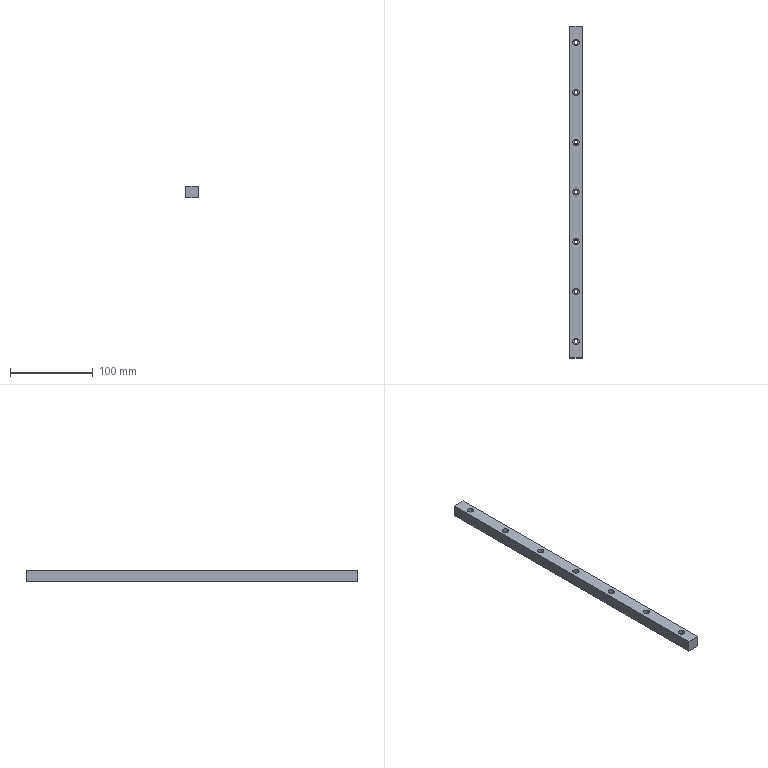Part | NX | 1 solid | 41 faces | box 15 x 400 x 14 mm | volume 81388 mm3 | cylinder 28 | plane 13 | commonest cylinder face diameters 4.5 x14 7.5 x12 8 x2
STEP:
#1=CARTESIAN_POINT('',(0.,-60.,0.));
#2=VERTEX_POINT('',#1);
#3=CARTESIAN_POINT('',(15.,-60.,0.));
#4=VERTEX_POINT('',#3);
#5=CARTESIAN_POINT('',(0.,-60.,0.));
#6=DIRECTION('',(1.,0.,0.));
#7=VECTOR('',#6,1000.);
#8=LINE('',#5,#7);
#9=EDGE_CURVE('',#2,#4,#8,.T.);
#10=ORIENTED_EDGE('',*,*,#9,.F.);
#11=CARTESIAN_POINT('',(0.,-60.,-14.));
#12=VERTEX_POINT('',#11);
#13=CARTESIAN_POINT('',(0.,-60.,0.));
#14=DIRECTION('',(0.,0.,1.));
#15=VECTOR('',#14,1000.);
#16=LINE('',#13,#15);
#17=EDGE_CURVE('',#12,#2,#16,.T.);
#18=ORIENTED_EDGE('',*,*,#17,.F.);
#19=CARTESIAN_POINT('',(15.,-60.,-14.));
#20=VERTEX_POINT('',#19);
#21=CARTESIAN_POINT('',(0.,-60.,-14.));
#22=DIRECTION('',(-1.,0.,0.));
#23=VECTOR('',#22,1000.);
#24=LINE('',#21,#23);
#25=EDGE_CURVE('',#20,#12,#24,.T.);
#26=ORIENTED_EDGE('',*,*,#25,.F.);
#27=CARTESIAN_POINT('',(15.,-60.,0.));
#28=DIRECTION('',(0.,0.,1.));
#29=VECTOR('',#28,1000.);
#30=LINE('',#27,#29);
#31=EDGE_CURVE('',#20,#4,#30,.T.);
#32=ORIENTED_EDGE('',*,*,#31,.T.);
#33=EDGE_LOOP('',(#10,#18,#26,#32));
#34=FACE_BOUND('',#33,.T.);
#35=CARTESIAN_POINT('',(76.5,-60.,-29.));
#36=DIRECTION('',(0.,-1.,0.));
#37=DIRECTION('',(0.,0.,-1.));
#38=AXIS2_PLACEMENT_3D('',#35,#36,#37);
#39=PLANE('',#38);
#40=ADVANCED_FACE('',(#34),#39,.T.);
#41=ORIENTED_EDGE('',*,*,#25,.T.);
#42=CARTESIAN_POINT('',(0.,340.,-14.));
#43=VERTEX_POINT('',#42);
#44=CARTESIAN_POINT('',(0.,0.,-14.));
#45=DIRECTION('',(0.,1.,0.));
#46=VECTOR('',#45,1000.);
#47=LINE('',#44,#46);
#48=EDGE_CURVE('',#12,#43,#47,.T.);
#49=ORIENTED_EDGE('',*,*,#48,.T.);
#50=CARTESIAN_POINT('',(15.,340.,-14.));
#51=VERTEX_POINT('',#50);
#52=CARTESIAN_POINT('',(0.,340.,-14.));
#53=DIRECTION('',(-1.,0.,0.));
#54=VECTOR('',#53,1000.);
#55=LINE('',#52,#54);
#56=EDGE_CURVE('',#51,#43,#55,.T.);
#57=ORIENTED_EDGE('',*,*,#56,.F.);
#58=CARTESIAN_POINT('',(15.,0.,-14.));
#59=DIRECTION('',(0.,-1.,0.));
#60=VECTOR('',#59,1000.);
#61=LINE('',#58,#60);
#62=EDGE_CURVE('',#51,#20,#61,.T.);
#63=ORIENTED_EDGE('',*,*,#62,.T.);
#64=EDGE_LOOP('',(#41,#49,#57,#63));
#65=FACE_BOUND('',#64,.T.);
#66=CARTESIAN_POINT('',(5.25,20.,-14.));
#67=VERTEX_POINT('',#66);
#68=CARTESIAN_POINT('',(9.75,20.,-14.));
#69=VERTEX_POINT('',#68);
#70=CARTESIAN_POINT('',(7.5,20.,-14.));
#71=DIRECTION('',(0.,0.,1.));
#72=DIRECTION('',(-1.,0.,0.));
#73=AXIS2_PLACEMENT_3D('',#70,#71,#72);
#74=CIRCLE('',#73,2.25);
#75=EDGE_CURVE('',#67,#69,#74,.T.);
#76=ORIENTED_EDGE('',*,*,#75,.T.);
#77=CARTESIAN_POINT('',(7.5,20.,-14.));
#78=DIRECTION('',(0.,0.,1.));
#79=DIRECTION('',(-1.,0.,0.));
#80=AXIS2_PLACEMENT_3D('',#77,#78,#79);
#81=CIRCLE('',#80,2.25);
#82=EDGE_CURVE('',#69,#67,#81,.T.);
#83=ORIENTED_EDGE('',*,*,#82,.T.);
#84=EDGE_LOOP('',(#76,#83));
#85=FACE_BOUND('',#84,.T.);
#86=CARTESIAN_POINT('',(5.25,320.,-14.));
#87=VERTEX_POINT('',#86);
#88=CARTESIAN_POINT('',(9.75,320.,-14.));
#89=VERTEX_POINT('',#88);
#90=CARTESIAN_POINT('',(7.5,320.,-14.));
#91=DIRECTION('',(0.,0.,1.));
#92=DIRECTION('',(-1.,0.,0.));
#93=AXIS2_PLACEMENT_3D('',#90,#91,#92);
#94=CIRCLE('',#93,2.25);
#95=EDGE_CURVE('',#87,#89,#94,.T.);
#96=ORIENTED_EDGE('',*,*,#95,.T.);
#97=CARTESIAN_POINT('',(7.5,320.,-14.));
#98=DIRECTION('',(0.,0.,1.));
#99=DIRECTION('',(-1.,0.,0.));
#100=AXIS2_PLACEMENT_3D('',#97,#98,#99);
#101=CIRCLE('',#100,2.25);
#102=EDGE_CURVE('',#89,#87,#101,.T.);
#103=ORIENTED_EDGE('',*,*,#102,.T.);
#104=EDGE_LOOP('',(#96,#103));
#105=FACE_BOUND('',#104,.T.);
#106=CARTESIAN_POINT('',(5.25,260.,-14.));
#107=VERTEX_POINT('',#106);
#108=CARTESIAN_POINT('',(9.75,260.,-14.));
#109=VERTEX_POINT('',#108);
#110=CARTESIAN_POINT('',(7.5,260.,-14.));
#111=DIRECTION('',(0.,0.,1.));
#112=DIRECTION('',(-1.,0.,0.));
#113=AXIS2_PLACEMENT_3D('',#110,#111,#112);
#114=CIRCLE('',#113,2.25);
#115=EDGE_CURVE('',#107,#109,#114,.T.);
#116=ORIENTED_EDGE('',*,*,#115,.T.);
#117=CARTESIAN_POINT('',(7.5,260.,-14.));
#118=DIRECTION('',(0.,0.,1.));
#119=DIRECTION('',(-1.,0.,0.));
#120=AXIS2_PLACEMENT_3D('',#117,#118,#119);
#121=CIRCLE('',#120,2.25);
#122=EDGE_CURVE('',#109,#107,#121,.T.);
#123=ORIENTED_EDGE('',*,*,#122,.T.);
#124=EDGE_LOOP('',(#116,#123));
#125=FACE_BOUND('',#124,.T.);
#126=CARTESIAN_POINT('',(9.75,200.,-14.));
#127=VERTEX_POINT('',#126);
#128=CARTESIAN_POINT('',(5.25,200.,-14.));
#129=VERTEX_POINT('',#128);
#130=CARTESIAN_POINT('',(7.5,200.,-14.));
#131=DIRECTION('',(0.,0.,1.));
#132=DIRECTION('',(-1.,0.,0.));
#133=AXIS2_PLACEMENT_3D('',#130,#131,#132);
#134=CIRCLE('',#133,2.25);
#135=EDGE_CURVE('',#127,#129,#134,.T.);
#136=ORIENTED_EDGE('',*,*,#135,.T.);
#137=CARTESIAN_POINT('',(7.5,200.,-14.));
#138=DIRECTION('',(0.,0.,1.));
#139=DIRECTION('',(-1.,0.,0.));
#140=AXIS2_PLACEMENT_3D('',#137,#138,#139);
#141=CIRCLE('',#140,2.25);
#142=EDGE_CURVE('',#129,#127,#141,.T.);
#143=ORIENTED_EDGE('',*,*,#142,.T.);
#144=EDGE_LOOP('',(#136,#143));
#145=FACE_BOUND('',#144,.T.);
#146=CARTESIAN_POINT('',(9.75,140.,-14.));
#147=VERTEX_POINT('',#146);
#148=CARTESIAN_POINT('',(5.25,140.,-14.));
#149=VERTEX_POINT('',#148);
#150=CARTESIAN_POINT('',(7.5,140.,-14.));
#151=DIRECTION('',(0.,0.,1.));
#152=DIRECTION('',(-1.,0.,0.));
#153=AXIS2_PLACEMENT_3D('',#150,#151,#152);
#154=CIRCLE('',#153,2.25);
#155=EDGE_CURVE('',#147,#149,#154,.T.);
#156=ORIENTED_EDGE('',*,*,#155,.T.);
#157=CARTESIAN_POINT('',(7.5,140.,-14.));
#158=DIRECTION('',(0.,0.,1.));
#159=DIRECTION('',(-1.,0.,0.));
#160=AXIS2_PLACEMENT_3D('',#157,#158,#159);
#161=CIRCLE('',#160,2.25);
#162=EDGE_CURVE('',#149,#147,#161,.T.);
#163=ORIENTED_EDGE('',*,*,#162,.T.);
#164=EDGE_LOOP('',(#156,#163));
#165=FACE_BOUND('',#164,.T.);
#166=CARTESIAN_POINT('',(9.75,80.,-14.));
#167=VERTEX_POINT('',#166);
#168=CARTESIAN_POINT('',(5.25,80.,-14.));
#169=VERTEX_POINT('',#168);
#170=CARTESIAN_POINT('',(7.5,80.,-14.));
#171=DIRECTION('',(0.,0.,1.));
#172=DIRECTION('',(-1.,0.,0.));
#173=AXIS2_PLACEMENT_3D('',#170,#171,#172);
#174=CIRCLE('',#173,2.25);
#175=EDGE_CURVE('',#167,#169,#174,.T.);
#176=ORIENTED_EDGE('',*,*,#175,.T.);
#177=CARTESIAN_POINT('',(7.5,80.,-14.));
#178=DIRECTION('',(0.,0.,1.));
#179=DIRECTION('',(-1.,0.,0.));
#180=AXIS2_PLACEMENT_3D('',#177,#178,#179);
#181=CIRCLE('',#180,2.25);
#182=EDGE_CURVE('',#169,#167,#181,.T.);
#183=ORIENTED_EDGE('',*,*,#182,.T.);
#184=EDGE_LOOP('',(#176,#183));
#185=FACE_BOUND('',#184,.T.);
#186=CARTESIAN_POINT('',(9.75,-40.,-14.));
#187=VERTEX_POINT('',#186);
#188=CARTESIAN_POINT('',(5.25,-40.,-14.));
#189=VERTEX_POINT('',#188);
#190=CARTESIAN_POINT('',(7.5,-40.,-14.));
#191=DIRECTION('',(0.,0.,1.));
#192=DIRECTION('',(1.,0.,0.));
#193=AXIS2_PLACEMENT_3D('',#190,#191,#192);
#194=CIRCLE('',#193,2.25);
#195=EDGE_CURVE('',#187,#189,#194,.T.);
#196=ORIENTED_EDGE('',*,*,#195,.T.);
#197=CARTESIAN_POINT('',(7.5,-40.,-14.));
#198=DIRECTION('',(0.,0.,1.));
#199=DIRECTION('',(1.,0.,0.));
#200=AXIS2_PLACEMENT_3D('',#197,#198,#199);
#201=CIRCLE('',#200,2.25);
#202=EDGE_CURVE('',#189,#187,#201,.T.);
#203=ORIENTED_EDGE('',*,*,#202,.T.);
#204=EDGE_LOOP('',(#196,#203));
#205=FACE_BOUND('',#204,.T.);
#206=CARTESIAN_POINT('',(15.,0.,-14.));
#207=DIRECTION('',(0.,0.,-1.));
#208=DIRECTION('',(0.,-1.,0.));
#209=AXIS2_PLACEMENT_3D('',#206,#207,#208);
#210=PLANE('',#209);
#211=ADVANCED_FACE('',(#65,#85,#105,#125,#145,#165,#185,#205),#210,.T.);
#212=ORIENTED_EDGE('',*,*,#17,.T.);
#213=CARTESIAN_POINT('',(0.,340.,0.));
#214=VERTEX_POINT('',#213);
#215=CARTESIAN_POINT('',(0.,0.,0.));
#216=DIRECTION('',(0.,1.,0.));
#217=VECTOR('',#216,1000.);
#218=LINE('',#215,#217);
#219=EDGE_CURVE('',#2,#214,#218,.T.);
#220=ORIENTED_EDGE('',*,*,#219,.T.);
#221=CARTESIAN_POINT('',(0.,340.,0.));
#222=DIRECTION('',(0.,0.,1.));
#223=VECTOR('',#222,1000.);
#224=LINE('',#221,#223);
#225=EDGE_CURVE('',#43,#214,#224,.T.);
#226=ORIENTED_EDGE('',*,*,#225,.F.);
#227=ORIENTED_EDGE('',*,*,#48,.F.);
#228=EDGE_LOOP('',(#212,#220,#226,#227));
#229=FACE_BOUND('',#228,.T.);
#230=CARTESIAN_POINT('',(0.,0.,-14.));
#231=DIRECTION('',(-1.,0.,0.));
#232=DIRECTION('',(0.,0.,1.));
#233=AXIS2_PLACEMENT_3D('',#230,#231,#232);
#234=PLANE('',#233);
#235=ADVANCED_FACE('',(#229),#234,.T.);
#236=ORIENTED_EDGE('',*,*,#9,.T.);
#237=CARTESIAN_POINT('',(15.,340.,0.));
#238=VERTEX_POINT('',#237);
#239=CARTESIAN_POINT('',(15.,0.,0.));
#240=DIRECTION('',(0.,1.,0.));
#241=VECTOR('',#240,1000.);
#242=LINE('',#239,#241);
#243=EDGE_CURVE('',#4,#238,#242,.T.);
#244=ORIENTED_EDGE('',*,*,#243,.T.);
#245=CARTESIAN_POINT('',(0.,340.,0.));
#246=DIRECTION('',(1.,0.,0.));
#247=VECTOR('',#246,1000.);
#248=LINE('',#245,#247);
#249=EDGE_CURVE('',#214,#238,#248,.T.);
#250=ORIENTED_EDGE('',*,*,#249,.F.);
#251=ORIENTED_EDGE('',*,*,#219,.F.);
#252=EDGE_LOOP('',(#236,#244,#250,#251));
#253=FACE_BOUND('',#252,.T.);
#254=CARTESIAN_POINT('',(11.25,20.,0.));
#255=VERTEX_POINT('',#254);
#256=CARTESIAN_POINT('',(3.75,20.,0.));
#257=VERTEX_POINT('',#256);
#258=CARTESIAN_POINT('',(7.5,20.,0.));
#259=DIRECTION('',(0.,0.,1.));
#260=DIRECTION('',(-1.,0.,0.));
#261=AXIS2_PLACEMENT_3D('',#258,#259,#260);
#262=CIRCLE('',#261,3.75);
#263=EDGE_CURVE('',#255,#257,#262,.T.);
#264=ORIENTED_EDGE('',*,*,#263,.F.);
#265=CARTESIAN_POINT('',(7.5,20.,0.));
#266=DIRECTION('',(0.,0.,1.));
#267=DIRECTION('',(-1.,0.,0.));
#268=AXIS2_PLACEMENT_3D('',#265,#266,#267);
#269=CIRCLE('',#268,3.75);
#270=EDGE_CURVE('',#257,#255,#269,.T.);
#271=ORIENTED_EDGE('',*,*,#270,.F.);
#272=EDGE_LOOP('',(#264,#271));
#273=FACE_BOUND('',#272,.T.);
#274=CARTESIAN_POINT('',(11.25,320.,0.));
#275=VERTEX_POINT('',#274);
#276=CARTESIAN_POINT('',(3.75,320.,0.));
#277=VERTEX_POINT('',#276);
#278=CARTESIAN_POINT('',(7.5,320.,0.));
#279=DIRECTION('',(0.,0.,1.));
#280=DIRECTION('',(-1.,0.,0.));
#281=AXIS2_PLACEMENT_3D('',#278,#279,#280);
#282=CIRCLE('',#281,3.75);
#283=EDGE_CURVE('',#275,#277,#282,.T.);
#284=ORIENTED_EDGE('',*,*,#283,.F.);
#285=CARTESIAN_POINT('',(7.5,320.,0.));
#286=DIRECTION('',(0.,0.,1.));
#287=DIRECTION('',(-1.,0.,0.));
#288=AXIS2_PLACEMENT_3D('',#285,#286,#287);
#289=CIRCLE('',#288,3.75);
#290=EDGE_CURVE('',#277,#275,#289,.T.);
#291=ORIENTED_EDGE('',*,*,#290,.F.);
#292=EDGE_LOOP('',(#284,#291));
#293=FACE_BOUND('',#292,.T.);
#294=CARTESIAN_POINT('',(11.25,260.,0.));
#295=VERTEX_POINT('',#294);
#296=CARTESIAN_POINT('',(3.75,260.,0.));
#297=VERTEX_POINT('',#296);
#298=CARTESIAN_POINT('',(7.5,260.,0.));
#299=DIRECTION('',(0.,0.,1.));
#300=DIRECTION('',(-1.,0.,0.));
#301=AXIS2_PLACEMENT_3D('',#298,#299,#300);
#302=CIRCLE('',#301,3.75);
#303=EDGE_CURVE('',#295,#297,#302,.T.);
#304=ORIENTED_EDGE('',*,*,#303,.F.);
#305=CARTESIAN_POINT('',(7.5,260.,0.));
#306=DIRECTION('',(0.,0.,1.));
#307=DIRECTION('',(-1.,0.,0.));
#308=AXIS2_PLACEMENT_3D('',#305,#306,#307);
#309=CIRCLE('',#308,3.75);
#310=EDGE_CURVE('',#297,#295,#309,.T.);
#311=ORIENTED_EDGE('',*,*,#310,.F.);
#312=EDGE_LOOP('',(#304,#311));
#313=FACE_BOUND('',#312,.T.);
#314=CARTESIAN_POINT('',(11.25,200.,0.));
#315=VERTEX_POINT('',#314);
#316=CARTESIAN_POINT('',(3.75,200.,0.));
#317=VERTEX_POINT('',#316);
#318=CARTESIAN_POINT('',(7.5,200.,0.));
#319=DIRECTION('',(0.,0.,1.));
#320=DIRECTION('',(-1.,0.,0.));
#321=AXIS2_PLACEMENT_3D('',#318,#319,#320);
#322=CIRCLE('',#321,3.75);
#323=EDGE_CURVE('',#315,#317,#322,.T.);
#324=ORIENTED_EDGE('',*,*,#323,.F.);
#325=CARTESIAN_POINT('',(7.5,200.,0.));
#326=DIRECTION('',(0.,0.,1.));
#327=DIRECTION('',(-1.,0.,0.));
#328=AXIS2_PLACEMENT_3D('',#325,#326,#327);
#329=CIRCLE('',#328,3.75);
#330=EDGE_CURVE('',#317,#315,#329,.T.);
#331=ORIENTED_EDGE('',*,*,#330,.F.);
#332=EDGE_LOOP('',(#324,#331));
#333=FACE_BOUND('',#332,.T.);
#334=CARTESIAN_POINT('',(11.25,140.,0.));
#335=VERTEX_POINT('',#334);
#336=CARTESIAN_POINT('',(3.75,140.,0.));
#337=VERTEX_POINT('',#336);
#338=CARTESIAN_POINT('',(7.5,140.,0.));
#339=DIRECTION('',(0.,0.,1.));
#340=DIRECTION('',(-1.,0.,0.));
#341=AXIS2_PLACEMENT_3D('',#338,#339,#340);
#342=CIRCLE('',#341,3.75);
#343=EDGE_CURVE('',#335,#337,#342,.T.);
#344=ORIENTED_EDGE('',*,*,#343,.F.);
#345=CARTESIAN_POINT('',(7.5,140.,0.));
#346=DIRECTION('',(0.,0.,1.));
#347=DIRECTION('',(-1.,0.,0.));
#348=AXIS2_PLACEMENT_3D('',#345,#346,#347);
#349=CIRCLE('',#348,3.75);
#350=EDGE_CURVE('',#337,#335,#349,.T.);
#351=ORIENTED_EDGE('',*,*,#350,.F.);
#352=EDGE_LOOP('',(#344,#351));
#353=FACE_BOUND('',#352,.T.);
#354=CARTESIAN_POINT('',(11.25,80.,0.));
#355=VERTEX_POINT('',#354);
#356=CARTESIAN_POINT('',(3.75,80.,0.));
#357=VERTEX_POINT('',#356);
#358=CARTESIAN_POINT('',(7.5,80.,0.));
#359=DIRECTION('',(0.,0.,1.));
#360=DIRECTION('',(-1.,0.,0.));
#361=AXIS2_PLACEMENT_3D('',#358,#359,#360);
#362=CIRCLE('',#361,3.75);
#363=EDGE_CURVE('',#355,#357,#362,.T.);
#364=ORIENTED_EDGE('',*,*,#363,.F.);
#365=CARTESIAN_POINT('',(7.5,80.,0.));
#366=DIRECTION('',(0.,0.,1.));
#367=DIRECTION('',(-1.,0.,0.));
#368=AXIS2_PLACEMENT_3D('',#365,#366,#367);
#369=CIRCLE('',#368,3.75);
#370=EDGE_CURVE('',#357,#355,#369,.T.);
#371=ORIENTED_EDGE('',*,*,#370,.F.);
#372=EDGE_LOOP('',(#364,#371));
#373=FACE_BOUND('',#372,.T.);
#374=CARTESIAN_POINT('',(3.5,-40.,0.));
#375=VERTEX_POINT('',#374);
#376=CARTESIAN_POINT('',(11.5,-40.,0.));
#377=VERTEX_POINT('',#376);
#378=CARTESIAN_POINT('',(7.5,-40.,0.));
#379=DIRECTION('',(0.,0.,1.));
#380=DIRECTION('',(1.,0.,0.));
#381=AXIS2_PLACEMENT_3D('',#378,#379,#380);
#382=CIRCLE('',#381,4.);
#383=EDGE_CURVE('',#375,#377,#382,.T.);
#384=ORIENTED_EDGE('',*,*,#383,.F.);
#385=CARTESIAN_POINT('',(7.5,-40.,0.));
#386=DIRECTION('',(0.,0.,1.));
#387=DIRECTION('',(1.,0.,0.));
#388=AXIS2_PLACEMENT_3D('',#385,#386,#387);
#389=CIRCLE('',#388,4.);
#390=EDGE_CURVE('',#377,#375,#389,.T.);
#391=ORIENTED_EDGE('',*,*,#390,.F.);
#392=EDGE_LOOP('',(#384,#391));
#393=FACE_BOUND('',#392,.T.);
#394=CARTESIAN_POINT('',(0.,0.,0.));
#395=DIRECTION('',(0.,0.,1.));
#396=DIRECTION('',(1.,0.,0.));
#397=AXIS2_PLACEMENT_3D('',#394,#395,#396);
#398=PLANE('',#397);
#399=ADVANCED_FACE('',(#253,#273,#293,#313,#333,#353,#373,#393),#398,.T.);
#400=ORIENTED_EDGE('',*,*,#31,.F.);
#401=ORIENTED_EDGE('',*,*,#62,.F.);
#402=CARTESIAN_POINT('',(15.,340.,0.));
#403=DIRECTION('',(0.,0.,-1.));
#404=VECTOR('',#403,1000.);
#405=LINE('',#402,#404);
#406=EDGE_CURVE('',#238,#51,#405,.T.);
#407=ORIENTED_EDGE('',*,*,#406,.F.);
#408=ORIENTED_EDGE('',*,*,#243,.F.);
#409=EDGE_LOOP('',(#400,#401,#407,#408));
#410=FACE_BOUND('',#409,.T.);
#411=CARTESIAN_POINT('',(15.,0.,0.));
#412=DIRECTION('',(1.,0.,0.));
#413=DIRECTION('',(0.,1.,0.));
#414=AXIS2_PLACEMENT_3D('',#411,#412,#413);
#415=PLANE('',#414);
#416=ADVANCED_FACE('',(#410),#415,.T.);
#417=ORIENTED_EDGE('',*,*,#249,.T.);
#418=ORIENTED_EDGE('',*,*,#406,.T.);
#419=ORIENTED_EDGE('',*,*,#56,.T.);
#420=ORIENTED_EDGE('',*,*,#225,.T.);
#421=EDGE_LOOP('',(#417,#418,#419,#420));
#422=FACE_BOUND('',#421,.T.);
#423=CARTESIAN_POINT('',(0.,340.,0.));
#424=DIRECTION('',(0.,1.,0.));
#425=DIRECTION('',(1.,0.,0.));
#426=AXIS2_PLACEMENT_3D('',#423,#424,#425);
#427=PLANE('',#426);
#428=ADVANCED_FACE('',(#422),#427,.T.);
#429=CARTESIAN_POINT('',(9.75,20.,-5.3));
#430=VERTEX_POINT('',#429);
#431=CARTESIAN_POINT('',(5.25,20.,-5.3));
#432=VERTEX_POINT('',#431);
#433=CARTESIAN_POINT('',(7.5,20.,-5.3));
#434=DIRECTION('',(0.,0.,1.));
#435=DIRECTION('',(1.,0.,0.));
#436=AXIS2_PLACEMENT_3D('',#433,#434,#435);
#437=CIRCLE('',#436,2.25);
#438=EDGE_CURVE('',#430,#432,#437,.T.);
#439=ORIENTED_EDGE('',*,*,#438,.T.);
#440=CARTESIAN_POINT('',(5.25,20.,-16.17));
#441=DIRECTION('',(0.,0.,1.));
#442=VECTOR('',#441,1000.);
#443=LINE('',#440,#442);
#444=EDGE_CURVE('',#432,#67,#443,.F.);
#445=ORIENTED_EDGE('',*,*,#444,.T.);
#446=ORIENTED_EDGE('',*,*,#82,.F.);
#447=CARTESIAN_POINT('',(9.75,20.,-16.17));
#448=DIRECTION('',(0.,0.,1.));
#449=VECTOR('',#448,1000.);
#450=LINE('',#447,#449);
#451=EDGE_CURVE('',#430,#69,#450,.F.);
#452=ORIENTED_EDGE('',*,*,#451,.F.);
#453=EDGE_LOOP('',(#439,#445,#446,#452));
#454=FACE_BOUND('',#453,.T.);
#455=CARTESIAN_POINT('',(7.5,20.,-16.17));
#456=DIRECTION('',(0.,0.,1.));
#457=DIRECTION('',(-1.,0.,0.));
#458=AXIS2_PLACEMENT_3D('',#455,#456,#457);
#459=CYLINDRICAL_SURFACE('',#458,2.25);
#460=ADVANCED_FACE('',(#454),#459,.F.);
#461=ORIENTED_EDGE('',*,*,#115,.F.);
#462=CARTESIAN_POINT('',(5.25,260.,-5.3));
#463=VERTEX_POINT('',#462);
#464=CARTESIAN_POINT('',(5.25,260.,-16.17));
#465=DIRECTION('',(0.,0.,1.));
#466=VECTOR('',#465,1000.);
#467=LINE('',#464,#466);
#468=EDGE_CURVE('',#463,#107,#467,.F.);
#469=ORIENTED_EDGE('',*,*,#468,.F.);
#470=CARTESIAN_POINT('',(9.75,260.,-5.3));
#471=VERTEX_POINT('',#470);
#472=CARTESIAN_POINT('',(7.5,260.,-5.3));
#473=DIRECTION('',(0.,0.,1.));
#474=DIRECTION('',(-1.,0.,0.));
#475=AXIS2_PLACEMENT_3D('',#472,#473,#474);
#476=CIRCLE('',#475,2.25);
#477=EDGE_CURVE('',#463,#471,#476,.T.);
#478=ORIENTED_EDGE('',*,*,#477,.T.);
#479=CARTESIAN_POINT('',(9.75,260.,-16.17));
#480=DIRECTION('',(0.,0.,1.));
#481=VECTOR('',#480,1000.);
#482=LINE('',#479,#481);
#483=EDGE_CURVE('',#471,#109,#482,.F.);
#484=ORIENTED_EDGE('',*,*,#483,.T.);
#485=EDGE_LOOP('',(#461,#469,#478,#484));
#486=FACE_BOUND('',#485,.T.);
#487=CARTESIAN_POINT('',(7.5,260.,-16.17));
#488=DIRECTION('',(0.,0.,1.));
#489=DIRECTION('',(-1.,0.,0.));
#490=AXIS2_PLACEMENT_3D('',#487,#488,#489);
#491=CYLINDRICAL_SURFACE('',#490,2.25);
#492=ADVANCED_FACE('',(#486),#491,.F.);
#493=CARTESIAN_POINT('',(11.25,20.,-5.3));
#494=VERTEX_POINT('',#493);
#495=CARTESIAN_POINT('',(3.75,20.,-5.3));
#496=VERTEX_POINT('',#495);
#497=CARTESIAN_POINT('',(7.5,20.,-5.3));
#498=DIRECTION('',(0.,0.,-1.));
#499=DIRECTION('',(-1.,0.,0.));
#500=AXIS2_PLACEMENT_3D('',#497,#498,#499);
#501=CIRCLE('',#500,3.75);
#502=EDGE_CURVE('',#494,#496,#501,.T.);
#503=ORIENTED_EDGE('',*,*,#502,.F.);
#504=CARTESIAN_POINT('',(7.5,20.,-5.3));
#505=DIRECTION('',(0.,0.,-1.));
#506=DIRECTION('',(-1.,0.,0.));
#507=AXIS2_PLACEMENT_3D('',#504,#505,#506);
#508=CIRCLE('',#507,3.75);
#509=EDGE_CURVE('',#496,#494,#508,.T.);
#510=ORIENTED_EDGE('',*,*,#509,.F.);
#511=EDGE_LOOP('',(#503,#510));
#512=FACE_BOUND('',#511,.T.);
#513=ORIENTED_EDGE('',*,*,#438,.F.);
#514=CARTESIAN_POINT('',(7.5,20.,-5.3));
#515=DIRECTION('',(0.,0.,1.));
#516=DIRECTION('',(1.,0.,0.));
#517=AXIS2_PLACEMENT_3D('',#514,#515,#516);
#518=CIRCLE('',#517,2.25);
#519=EDGE_CURVE('',#432,#430,#518,.T.);
#520=ORIENTED_EDGE('',*,*,#519,.F.);
#521=EDGE_LOOP('',(#513,#520));
#522=FACE_BOUND('',#521,.T.);
#523=CARTESIAN_POINT('',(7.5,20.,-5.3));
#524=DIRECTION('',(0.,0.,1.));
#525=DIRECTION('',(1.,0.,0.));
#526=AXIS2_PLACEMENT_3D('',#523,#524,#525);
#527=PLANE('',#526);
#528=ADVANCED_FACE('',(#512,#522),#527,.T.);
#529=ORIENTED_EDGE('',*,*,#502,.T.);
#530=CARTESIAN_POINT('',(3.75,20.,-16.17));
#531=DIRECTION('',(0.,0.,1.));
#532=VECTOR('',#531,1000.);
#533=LINE('',#530,#532);
#534=EDGE_CURVE('',#257,#496,#533,.F.);
#535=ORIENTED_EDGE('',*,*,#534,.F.);
#536=ORIENTED_EDGE('',*,*,#270,.T.);
#537=CARTESIAN_POINT('',(11.25,20.,-16.17));
#538=DIRECTION('',(0.,0.,1.));
#539=VECTOR('',#538,1000.);
#540=LINE('',#537,#539);
#541=EDGE_CURVE('',#255,#494,#540,.F.);
#542=ORIENTED_EDGE('',*,*,#541,.T.);
#543=EDGE_LOOP('',(#529,#535,#536,#542));
#544=FACE_BOUND('',#543,.T.);
#545=CARTESIAN_POINT('',(7.5,20.,-16.17));
#546=DIRECTION('',(0.,0.,1.));
#547=DIRECTION('',(-1.,0.,0.));
#548=AXIS2_PLACEMENT_3D('',#545,#546,#547);
#549=CYLINDRICAL_SURFACE('',#548,3.75);
#550=ADVANCED_FACE('',(#544),#549,.F.);
#551=ORIENTED_EDGE('',*,*,#323,.T.);
#552=CARTESIAN_POINT('',(3.75,200.,-5.3));
#553=VERTEX_POINT('',#552);
#554=CARTESIAN_POINT('',(3.75,200.,-16.17));
#555=DIRECTION('',(0.,0.,1.));
#556=VECTOR('',#555,1000.);
#557=LINE('',#554,#556);
#558=EDGE_CURVE('',#317,#553,#557,.F.);
#559=ORIENTED_EDGE('',*,*,#558,.T.);
#560=CARTESIAN_POINT('',(11.25,200.,-5.3));
#561=VERTEX_POINT('',#560);
#562=CARTESIAN_POINT('',(7.5,200.,-5.3));
#563=DIRECTION('',(0.,0.,-1.));
#564=DIRECTION('',(-1.,0.,0.));
#565=AXIS2_PLACEMENT_3D('',#562,#563,#564);
#566=CIRCLE('',#565,3.75);
#567=EDGE_CURVE('',#553,#561,#566,.T.);
#568=ORIENTED_EDGE('',*,*,#567,.T.);
#569=CARTESIAN_POINT('',(11.25,200.,-16.17));
#570=DIRECTION('',(0.,0.,1.));
#571=VECTOR('',#570,1000.);
#572=LINE('',#569,#571);
#573=EDGE_CURVE('',#315,#561,#572,.F.);
#574=ORIENTED_EDGE('',*,*,#573,.F.);
#575=EDGE_LOOP('',(#551,#559,#568,#574));
#576=FACE_BOUND('',#575,.T.);
#577=CARTESIAN_POINT('',(7.5,200.,-16.17));
#578=DIRECTION('',(0.,0.,1.));
#579=DIRECTION('',(-1.,0.,0.));
#580=AXIS2_PLACEMENT_3D('',#577,#578,#579);
#581=CYLINDRICAL_SURFACE('',#580,3.75);
#582=ADVANCED_FACE('',(#576),#581,.F.);
#583=CARTESIAN_POINT('',(9.75,80.,-5.3));
#584=VERTEX_POINT('',#583);
#585=CARTESIAN_POINT('',(5.25,80.,-5.3));
#586=VERTEX_POINT('',#585);
#587=CARTESIAN_POINT('',(7.5,80.,-5.3));
#588=DIRECTION('',(0.,0.,1.));
#589=DIRECTION('',(-1.,0.,0.));
#590=AXIS2_PLACEMENT_3D('',#587,#588,#589);
#591=CIRCLE('',#590,2.25);
#592=EDGE_CURVE('',#584,#586,#591,.T.);
#593=ORIENTED_EDGE('',*,*,#592,.T.);
#594=CARTESIAN_POINT('',(5.25,80.,-16.17));
#595=DIRECTION('',(0.,0.,1.));
#596=VECTOR('',#595,1000.);
#597=LINE('',#594,#596);
#598=EDGE_CURVE('',#586,#169,#597,.F.);
#599=ORIENTED_EDGE('',*,*,#598,.T.);
#600=ORIENTED_EDGE('',*,*,#175,.F.);
#601=CARTESIAN_POINT('',(9.75,80.,-16.17));
#602=DIRECTION('',(0.,0.,1.));
#603=VECTOR('',#602,1000.);
#604=LINE('',#601,#603);
#605=EDGE_CURVE('',#584,#167,#604,.F.);
#606=ORIENTED_EDGE('',*,*,#605,.F.);
#607=EDGE_LOOP('',(#593,#599,#600,#606));
#608=FACE_BOUND('',#607,.T.);
#609=CARTESIAN_POINT('',(7.5,80.,-16.17));
#610=DIRECTION('',(0.,0.,1.));
#611=DIRECTION('',(-1.,0.,0.));
#612=AXIS2_PLACEMENT_3D('',#609,#610,#611);
#613=CYLINDRICAL_SURFACE('',#612,2.25);
#614=ADVANCED_FACE('',(#608),#613,.F.);
#615=CARTESIAN_POINT('',(3.75,320.,-5.3));
#616=VERTEX_POINT('',#615);
#617=CARTESIAN_POINT('',(11.25,320.,-5.3));
#618=VERTEX_POINT('',#617);
#619=CARTESIAN_POINT('',(7.5,320.,-5.3));
#620=DIRECTION('',(0.,0.,-1.));
#621=DIRECTION('',(-1.,0.,0.));
#622=AXIS2_PLACEMENT_3D('',#619,#620,#621);
#623=CIRCLE('',#622,3.75);
#624=EDGE_CURVE('',#616,#618,#623,.T.);
#625=ORIENTED_EDGE('',*,*,#624,.F.);
#626=CARTESIAN_POINT('',(7.5,320.,-5.3));
#627=DIRECTION('',(0.,0.,-1.));
#628=DIRECTION('',(-1.,0.,0.));
#629=AXIS2_PLACEMENT_3D('',#626,#627,#628);
#630=CIRCLE('',#629,3.75);
#631=EDGE_CURVE('',#618,#616,#630,.T.);
#632=ORIENTED_EDGE('',*,*,#631,.F.);
#633=EDGE_LOOP('',(#625,#632));
#634=FACE_BOUND('',#633,.T.);
#635=CARTESIAN_POINT('',(5.25,320.,-5.3));
#636=VERTEX_POINT('',#635);
#637=CARTESIAN_POINT('',(9.75,320.,-5.3));
#638=VERTEX_POINT('',#637);
#639=CARTESIAN_POINT('',(7.5,320.,-5.3));
#640=DIRECTION('',(0.,0.,1.));
#641=DIRECTION('',(1.,0.,0.));
#642=AXIS2_PLACEMENT_3D('',#639,#640,#641);
#643=CIRCLE('',#642,2.25);
#644=EDGE_CURVE('',#636,#638,#643,.T.);
#645=ORIENTED_EDGE('',*,*,#644,.F.);
#646=CARTESIAN_POINT('',(7.5,320.,-5.3));
#647=DIRECTION('',(0.,0.,1.));
#648=DIRECTION('',(1.,0.,0.));
#649=AXIS2_PLACEMENT_3D('',#646,#647,#648);
#650=CIRCLE('',#649,2.25);
#651=EDGE_CURVE('',#638,#636,#650,.T.);
#652=ORIENTED_EDGE('',*,*,#651,.F.);
#653=EDGE_LOOP('',(#645,#652));
#654=FACE_BOUND('',#653,.T.);
#655=CARTESIAN_POINT('',(7.5,320.,-5.3));
#656=DIRECTION('',(0.,0.,1.));
#657=DIRECTION('',(1.,0.,0.));
#658=AXIS2_PLACEMENT_3D('',#655,#656,#657);
#659=PLANE('',#658);
#660=ADVANCED_FACE('',(#634,#654),#659,.T.);
#661=CARTESIAN_POINT('',(3.75,80.,-5.3));
#662=VERTEX_POINT('',#661);
#663=CARTESIAN_POINT('',(11.25,80.,-5.3));
#664=VERTEX_POINT('',#663);
#665=CARTESIAN_POINT('',(7.5,80.,-5.3));
#666=DIRECTION('',(0.,0.,-1.));
#667=DIRECTION('',(-1.,0.,0.));
#668=AXIS2_PLACEMENT_3D('',#665,#666,#667);
#669=CIRCLE('',#668,3.75);
#670=EDGE_CURVE('',#662,#664,#669,.T.);
#671=ORIENTED_EDGE('',*,*,#670,.F.);
#672=CARTESIAN_POINT('',(7.5,80.,-5.3));
#673=DIRECTION('',(0.,0.,-1.));
#674=DIRECTION('',(-1.,0.,0.));
#675=AXIS2_PLACEMENT_3D('',#672,#673,#674);
#676=CIRCLE('',#675,3.75);
#677=EDGE_CURVE('',#664,#662,#676,.T.);
#678=ORIENTED_EDGE('',*,*,#677,.F.);
#679=EDGE_LOOP('',(#671,#678));
#680=FACE_BOUND('',#679,.T.);
#681=ORIENTED_EDGE('',*,*,#592,.F.);
#682=CARTESIAN_POINT('',(7.5,80.,-5.3));
#683=DIRECTION('',(0.,0.,1.));
#684=DIRECTION('',(-1.,0.,0.));
#685=AXIS2_PLACEMENT_3D('',#682,#683,#684);
#686=CIRCLE('',#685,2.25);
#687=EDGE_CURVE('',#586,#584,#686,.T.);
#688=ORIENTED_EDGE('',*,*,#687,.F.);
#689=EDGE_LOOP('',(#681,#688));
#690=FACE_BOUND('',#689,.T.);
#691=CARTESIAN_POINT('',(7.5,80.,-5.3));
#692=DIRECTION('',(0.,0.,1.));
#693=DIRECTION('',(1.,0.,0.));
#694=AXIS2_PLACEMENT_3D('',#691,#692,#693);
#695=PLANE('',#694);
#696=ADVANCED_FACE('',(#680,#690),#695,.T.);
#697=ORIENTED_EDGE('',*,*,#363,.T.);
#698=CARTESIAN_POINT('',(3.75,80.,-16.17));
#699=DIRECTION('',(0.,0.,1.));
#700=VECTOR('',#699,1000.);
#701=LINE('',#698,#700);
#702=EDGE_CURVE('',#357,#662,#701,.F.);
#703=ORIENTED_EDGE('',*,*,#702,.T.);
#704=ORIENTED_EDGE('',*,*,#670,.T.);
#705=CARTESIAN_POINT('',(11.25,80.,-16.17));
#706=DIRECTION('',(0.,0.,1.));
#707=VECTOR('',#706,1000.);
#708=LINE('',#705,#707);
#709=EDGE_CURVE('',#355,#664,#708,.F.);
#710=ORIENTED_EDGE('',*,*,#709,.F.);
#711=EDGE_LOOP('',(#697,#703,#704,#710));
#712=FACE_BOUND('',#711,.T.);
#713=CARTESIAN_POINT('',(7.5,80.,-16.17));
#714=DIRECTION('',(0.,0.,1.));
#715=DIRECTION('',(-1.,0.,0.));
#716=AXIS2_PLACEMENT_3D('',#713,#714,#715);
#717=CYLINDRICAL_SURFACE('',#716,3.75);
#718=ADVANCED_FACE('',(#712),#717,.F.);
#719=CARTESIAN_POINT('',(3.75,260.,-5.3));
#720=VERTEX_POINT('',#719);
#721=CARTESIAN_POINT('',(11.25,260.,-5.3));
#722=VERTEX_POINT('',#721);
#723=CARTESIAN_POINT('',(7.5,260.,-5.3));
#724=DIRECTION('',(0.,0.,-1.));
#725=DIRECTION('',(-1.,0.,0.));
#726=AXIS2_PLACEMENT_3D('',#723,#724,#725);
#727=CIRCLE('',#726,3.75);
#728=EDGE_CURVE('',#720,#722,#727,.T.);
#729=ORIENTED_EDGE('',*,*,#728,.T.);
#730=CARTESIAN_POINT('',(11.25,260.,-16.17));
#731=DIRECTION('',(0.,0.,1.));
#732=VECTOR('',#731,1000.);
#733=LINE('',#730,#732);
#734=EDGE_CURVE('',#295,#722,#733,.F.);
#735=ORIENTED_EDGE('',*,*,#734,.F.);
#736=ORIENTED_EDGE('',*,*,#303,.T.);
#737=CARTESIAN_POINT('',(3.75,260.,-16.17));
#738=DIRECTION('',(0.,0.,1.));
#739=VECTOR('',#738,1000.);
#740=LINE('',#737,#739);
#741=EDGE_CURVE('',#297,#720,#740,.F.);
#742=ORIENTED_EDGE('',*,*,#741,.T.);
#743=EDGE_LOOP('',(#729,#735,#736,#742));
#744=FACE_BOUND('',#743,.T.);
#745=CARTESIAN_POINT('',(7.5,260.,-16.17));
#746=DIRECTION('',(0.,0.,1.));
#747=DIRECTION('',(-1.,0.,0.));
#748=AXIS2_PLACEMENT_3D('',#745,#746,#747);
#749=CYLINDRICAL_SURFACE('',#748,3.75);
#750=ADVANCED_FACE('',(#744),#749,.F.);
#751=CARTESIAN_POINT('',(5.25,140.,-5.3));
#752=VERTEX_POINT('',#751);
#753=CARTESIAN_POINT('',(9.75,140.,-5.3));
#754=VERTEX_POINT('',#753);
#755=CARTESIAN_POINT('',(7.5,140.,-5.3));
#756=DIRECTION('',(0.,0.,1.));
#757=DIRECTION('',(-1.,0.,0.));
#758=AXIS2_PLACEMENT_3D('',#755,#756,#757);
#759=CIRCLE('',#758,2.25);
#760=EDGE_CURVE('',#752,#754,#759,.T.);
#761=ORIENTED_EDGE('',*,*,#760,.T.);
#762=CARTESIAN_POINT('',(9.75,140.,-16.17));
#763=DIRECTION('',(0.,0.,1.));
#764=VECTOR('',#763,1000.);
#765=LINE('',#762,#764);
#766=EDGE_CURVE('',#147,#754,#765,.T.);
#767=ORIENTED_EDGE('',*,*,#766,.F.);
#768=ORIENTED_EDGE('',*,*,#162,.F.);
#769=CARTESIAN_POINT('',(5.25,140.,-16.17));
#770=DIRECTION('',(0.,0.,1.));
#771=VECTOR('',#770,1000.);
#772=LINE('',#769,#771);
#773=EDGE_CURVE('',#149,#752,#772,.T.);
#774=ORIENTED_EDGE('',*,*,#773,.T.);
#775=EDGE_LOOP('',(#761,#767,#768,#774));
#776=FACE_BOUND('',#775,.T.);
#777=CARTESIAN_POINT('',(7.5,140.,-16.17));
#778=DIRECTION('',(0.,0.,1.));
#779=DIRECTION('',(-1.,0.,0.));
#780=AXIS2_PLACEMENT_3D('',#777,#778,#779);
#781=CYLINDRICAL_SURFACE('',#780,2.25);
#782=ADVANCED_FACE('',(#776),#781,.F.);
#783=ORIENTED_EDGE('',*,*,#728,.F.);
#784=CARTESIAN_POINT('',(7.5,260.,-5.3));
#785=DIRECTION('',(0.,0.,-1.));
#786=DIRECTION('',(-1.,0.,0.));
#787=AXIS2_PLACEMENT_3D('',#784,#785,#786);
#788=CIRCLE('',#787,3.75);
#789=EDGE_CURVE('',#722,#720,#788,.T.);
#790=ORIENTED_EDGE('',*,*,#789,.F.);
#791=EDGE_LOOP('',(#783,#790));
#792=FACE_BOUND('',#791,.T.);
#793=ORIENTED_EDGE('',*,*,#477,.F.);
#794=CARTESIAN_POINT('',(7.5,260.,-5.3));
#795=DIRECTION('',(0.,0.,1.));
#796=DIRECTION('',(-1.,0.,0.));
#797=AXIS2_PLACEMENT_3D('',#794,#795,#796);
#798=CIRCLE('',#797,2.25);
#799=EDGE_CURVE('',#471,#463,#798,.T.);
#800=ORIENTED_EDGE('',*,*,#799,.F.);
#801=EDGE_LOOP('',(#793,#800));
#802=FACE_BOUND('',#801,.T.);
#803=CARTESIAN_POINT('',(7.5,260.,-5.3));
#804=DIRECTION('',(0.,0.,1.));
#805=DIRECTION('',(1.,0.,0.));
#806=AXIS2_PLACEMENT_3D('',#803,#804,#805);
#807=PLANE('',#806);
#808=ADVANCED_FACE('',(#792,#802),#807,.T.);
#809=CARTESIAN_POINT('',(11.25,140.,-5.3));
#810=VERTEX_POINT('',#809);
#811=CARTESIAN_POINT('',(3.75,140.,-5.3));
#812=VERTEX_POINT('',#811);
#813=CARTESIAN_POINT('',(7.5,140.,-5.3));
#814=DIRECTION('',(0.,0.,-1.));
#815=DIRECTION('',(-1.,0.,0.));
#816=AXIS2_PLACEMENT_3D('',#813,#814,#815);
#817=CIRCLE('',#816,3.75);
#818=EDGE_CURVE('',#810,#812,#817,.T.);
#819=ORIENTED_EDGE('',*,*,#818,.F.);
#820=CARTESIAN_POINT('',(7.5,140.,-5.3));
#821=DIRECTION('',(0.,0.,-1.));
#822=DIRECTION('',(-1.,0.,0.));
#823=AXIS2_PLACEMENT_3D('',#820,#821,#822);
#824=CIRCLE('',#823,3.75);
#825=EDGE_CURVE('',#812,#810,#824,.T.);
#826=ORIENTED_EDGE('',*,*,#825,.F.);
#827=EDGE_LOOP('',(#819,#826));
#828=FACE_BOUND('',#827,.T.);
#829=ORIENTED_EDGE('',*,*,#760,.F.);
#830=CARTESIAN_POINT('',(7.5,140.,-5.3));
#831=DIRECTION('',(0.,0.,1.));
#832=DIRECTION('',(-1.,0.,0.));
#833=AXIS2_PLACEMENT_3D('',#830,#831,#832);
#834=CIRCLE('',#833,2.25);
#835=EDGE_CURVE('',#754,#752,#834,.T.);
#836=ORIENTED_EDGE('',*,*,#835,.F.);
#837=EDGE_LOOP('',(#829,#836));
#838=FACE_BOUND('',#837,.T.);
#839=CARTESIAN_POINT('',(7.5,140.,-5.3));
#840=DIRECTION('',(0.,0.,1.));
#841=DIRECTION('',(1.,0.,0.));
#842=AXIS2_PLACEMENT_3D('',#839,#840,#841);
#843=PLANE('',#842);
#844=ADVANCED_FACE('',(#828,#838),#843,.T.);
#845=ORIENTED_EDGE('',*,*,#343,.T.);
#846=CARTESIAN_POINT('',(3.75,140.,-16.17));
#847=DIRECTION('',(0.,0.,1.));
#848=VECTOR('',#847,1000.);
#849=LINE('',#846,#848);
#850=EDGE_CURVE('',#337,#812,#849,.F.);
#851=ORIENTED_EDGE('',*,*,#850,.T.);
#852=ORIENTED_EDGE('',*,*,#825,.T.);
#853=CARTESIAN_POINT('',(11.25,140.,-16.17));
#854=DIRECTION('',(0.,0.,1.));
#855=VECTOR('',#854,1000.);
#856=LINE('',#853,#855);
#857=EDGE_CURVE('',#335,#810,#856,.F.);
#858=ORIENTED_EDGE('',*,*,#857,.F.);
#859=EDGE_LOOP('',(#845,#851,#852,#858));
#860=FACE_BOUND('',#859,.T.);
#861=CARTESIAN_POINT('',(7.5,140.,-16.17));
#862=DIRECTION('',(0.,0.,1.));
#863=DIRECTION('',(-1.,0.,0.));
#864=AXIS2_PLACEMENT_3D('',#861,#862,#863);
#865=CYLINDRICAL_SURFACE('',#864,3.75);
#866=ADVANCED_FACE('',(#860),#865,.F.);
#867=ORIENTED_EDGE('',*,*,#283,.T.);
#868=CARTESIAN_POINT('',(3.75,320.,-16.17));
#869=DIRECTION('',(0.,0.,1.));
#870=VECTOR('',#869,1000.);
#871=LINE('',#868,#870);
#872=EDGE_CURVE('',#277,#616,#871,.F.);
#873=ORIENTED_EDGE('',*,*,#872,.T.);
#874=ORIENTED_EDGE('',*,*,#624,.T.);
#875=CARTESIAN_POINT('',(11.25,320.,-16.17));
#876=DIRECTION('',(0.,0.,1.));
#877=VECTOR('',#876,1000.);
#878=LINE('',#875,#877);
#879=EDGE_CURVE('',#275,#618,#878,.F.);
#880=ORIENTED_EDGE('',*,*,#879,.F.);
#881=EDGE_LOOP('',(#867,#873,#874,#880));
#882=FACE_BOUND('',#881,.T.);
#883=CARTESIAN_POINT('',(7.5,320.,-16.17));
#884=DIRECTION('',(0.,0.,1.));
#885=DIRECTION('',(-1.,0.,0.));
#886=AXIS2_PLACEMENT_3D('',#883,#884,#885);
#887=CYLINDRICAL_SURFACE('',#886,3.75);
#888=ADVANCED_FACE('',(#882),#887,.F.);
#889=CARTESIAN_POINT('',(9.75,200.,-5.3));
#890=VERTEX_POINT('',#889);
#891=CARTESIAN_POINT('',(5.25,200.,-5.3));
#892=VERTEX_POINT('',#891);
#893=CARTESIAN_POINT('',(7.5,200.,-5.3));
#894=DIRECTION('',(0.,0.,1.));
#895=DIRECTION('',(-1.,0.,0.));
#896=AXIS2_PLACEMENT_3D('',#893,#894,#895);
#897=CIRCLE('',#896,2.25);
#898=EDGE_CURVE('',#890,#892,#897,.T.);
#899=ORIENTED_EDGE('',*,*,#898,.T.);
#900=CARTESIAN_POINT('',(5.25,200.,-16.17));
#901=DIRECTION('',(0.,0.,1.));
#902=VECTOR('',#901,1000.);
#903=LINE('',#900,#902);
#904=EDGE_CURVE('',#892,#129,#903,.F.);
#905=ORIENTED_EDGE('',*,*,#904,.T.);
#906=ORIENTED_EDGE('',*,*,#135,.F.);
#907=CARTESIAN_POINT('',(9.75,200.,-16.17));
#908=DIRECTION('',(0.,0.,1.));
#909=VECTOR('',#908,1000.);
#910=LINE('',#907,#909);
#911=EDGE_CURVE('',#890,#127,#910,.F.);
#912=ORIENTED_EDGE('',*,*,#911,.F.);
#913=EDGE_LOOP('',(#899,#905,#906,#912));
#914=FACE_BOUND('',#913,.T.);
#915=CARTESIAN_POINT('',(7.5,200.,-16.17));
#916=DIRECTION('',(0.,0.,1.));
#917=DIRECTION('',(-1.,0.,0.));
#918=AXIS2_PLACEMENT_3D('',#915,#916,#917);
#919=CYLINDRICAL_SURFACE('',#918,2.25);
#920=ADVANCED_FACE('',(#914),#919,.F.);
#921=ORIENTED_EDGE('',*,*,#644,.T.);
#922=CARTESIAN_POINT('',(9.75,320.,-16.17));
#923=DIRECTION('',(0.,0.,1.));
#924=VECTOR('',#923,1000.);
#925=LINE('',#922,#924);
#926=EDGE_CURVE('',#638,#89,#925,.F.);
#927=ORIENTED_EDGE('',*,*,#926,.T.);
#928=ORIENTED_EDGE('',*,*,#95,.F.);
#929=CARTESIAN_POINT('',(5.25,320.,-16.17));
#930=DIRECTION('',(0.,0.,1.));
#931=VECTOR('',#930,1000.);
#932=LINE('',#929,#931);
#933=EDGE_CURVE('',#636,#87,#932,.F.);
#934=ORIENTED_EDGE('',*,*,#933,.F.);
#935=EDGE_LOOP('',(#921,#927,#928,#934));
#936=FACE_BOUND('',#935,.T.);
#937=CARTESIAN_POINT('',(7.5,320.,-16.17));
#938=DIRECTION('',(0.,0.,1.));
#939=DIRECTION('',(-1.,0.,0.));
#940=AXIS2_PLACEMENT_3D('',#937,#938,#939);
#941=CYLINDRICAL_SURFACE('',#940,2.25);
#942=ADVANCED_FACE('',(#936),#941,.F.);
#943=CARTESIAN_POINT('',(7.5,200.,-5.3));
#944=DIRECTION('',(0.,0.,-1.));
#945=DIRECTION('',(-1.,0.,0.));
#946=AXIS2_PLACEMENT_3D('',#943,#944,#945);
#947=CIRCLE('',#946,3.75);
#948=EDGE_CURVE('',#561,#553,#947,.T.);
#949=ORIENTED_EDGE('',*,*,#948,.F.);
#950=ORIENTED_EDGE('',*,*,#567,.F.);
#951=EDGE_LOOP('',(#949,#950));
#952=FACE_BOUND('',#951,.T.);
#953=ORIENTED_EDGE('',*,*,#898,.F.);
#954=CARTESIAN_POINT('',(7.5,200.,-5.3));
#955=DIRECTION('',(0.,0.,1.));
#956=DIRECTION('',(-1.,0.,0.));
#957=AXIS2_PLACEMENT_3D('',#954,#955,#956);
#958=CIRCLE('',#957,2.25);
#959=EDGE_CURVE('',#892,#890,#958,.T.);
#960=ORIENTED_EDGE('',*,*,#959,.F.);
#961=EDGE_LOOP('',(#953,#960));
#962=FACE_BOUND('',#961,.T.);
#963=CARTESIAN_POINT('',(7.5,200.,-5.3));
#964=DIRECTION('',(0.,0.,1.));
#965=DIRECTION('',(1.,0.,0.));
#966=AXIS2_PLACEMENT_3D('',#963,#964,#965);
#967=PLANE('',#966);
#968=ADVANCED_FACE('',(#952,#962),#967,.T.);
#969=ORIENTED_EDGE('',*,*,#195,.F.);
#970=CARTESIAN_POINT('',(9.75,-40.,-4.5));
#971=VERTEX_POINT('',#970);
#972=CARTESIAN_POINT('',(9.75,-40.,-15.4));
#973=DIRECTION('',(0.,0.,1.));
#974=VECTOR('',#973,1000.);
#975=LINE('',#972,#974);
#976=EDGE_CURVE('',#187,#971,#975,.T.);
#977=ORIENTED_EDGE('',*,*,#976,.T.);
#978=CARTESIAN_POINT('',(5.25,-40.,-4.5));
#979=VERTEX_POINT('',#978);
#980=CARTESIAN_POINT('',(7.5,-40.,-4.5));
#981=DIRECTION('',(0.,0.,1.));
#982=DIRECTION('',(1.,0.,0.));
#983=AXIS2_PLACEMENT_3D('',#980,#981,#982);
#984=CIRCLE('',#983,2.25);
#985=EDGE_CURVE('',#971,#979,#984,.T.);
#986=ORIENTED_EDGE('',*,*,#985,.T.);
#987=CARTESIAN_POINT('',(5.25,-40.,-15.4));
#988=DIRECTION('',(0.,0.,1.));
#989=VECTOR('',#988,1000.);
#990=LINE('',#987,#989);
#991=EDGE_CURVE('',#189,#979,#990,.T.);
#992=ORIENTED_EDGE('',*,*,#991,.F.);
#993=EDGE_LOOP('',(#969,#977,#986,#992));
#994=FACE_BOUND('',#993,.T.);
#995=CARTESIAN_POINT('',(7.5,-40.,-15.4));
#996=DIRECTION('',(0.,0.,1.));
#997=DIRECTION('',(1.,0.,0.));
#998=AXIS2_PLACEMENT_3D('',#995,#996,#997);
#999=CYLINDRICAL_SURFACE('',#998,2.25);
#1000=ADVANCED_FACE('',(#994),#999,.F.);
#1001=CARTESIAN_POINT('',(3.5,-40.,-4.5));
#1002=VERTEX_POINT('',#1001);
#1003=CARTESIAN_POINT('',(11.5,-40.,-4.5));
#1004=VERTEX_POINT('',#1003);
#1005=CARTESIAN_POINT('',(7.5,-40.,-4.5));
#1006=DIRECTION('',(0.,0.,1.));
#1007=DIRECTION('',(1.,0.,0.));
#1008=AXIS2_PLACEMENT_3D('',#1005,#1006,#1007);
#1009=CIRCLE('',#1008,4.);
#1010=EDGE_CURVE('',#1002,#1004,#1009,.T.);
#1011=ORIENTED_EDGE('',*,*,#1010,.T.);
#1012=CARTESIAN_POINT('',(7.5,-40.,-4.5));
#1013=DIRECTION('',(0.,0.,1.));
#1014=DIRECTION('',(1.,0.,0.));
#1015=AXIS2_PLACEMENT_3D('',#1012,#1013,#1014);
#1016=CIRCLE('',#1015,4.);
#1017=EDGE_CURVE('',#1004,#1002,#1016,.T.);
#1018=ORIENTED_EDGE('',*,*,#1017,.T.);
#1019=EDGE_LOOP('',(#1011,#1018));
#1020=FACE_BOUND('',#1019,.T.);
#1021=CARTESIAN_POINT('',(7.5,-40.,-4.5));
#1022=DIRECTION('',(0.,0.,1.));
#1023=DIRECTION('',(1.,0.,0.));
#1024=AXIS2_PLACEMENT_3D('',#1021,#1022,#1023);
#1025=CIRCLE('',#1024,2.25);
#1026=EDGE_CURVE('',#979,#971,#1025,.T.);
#1027=ORIENTED_EDGE('',*,*,#1026,.F.);
#1028=ORIENTED_EDGE('',*,*,#985,.F.);
#1029=EDGE_LOOP('',(#1027,#1028));
#1030=FACE_BOUND('',#1029,.T.);
#1031=CARTESIAN_POINT('',(8.924,-22.23,-4.5));
#1032=DIRECTION('',(0.,0.,1.));
#1033=DIRECTION('',(1.,0.,0.));
#1034=AXIS2_PLACEMENT_3D('',#1031,#1032,#1033);
#1035=PLANE('',#1034);
#1036=ADVANCED_FACE('',(#1020,#1030),#1035,.T.);
#1037=ORIENTED_EDGE('',*,*,#1010,.F.);
#1038=CARTESIAN_POINT('',(3.5,-40.,0.));
#1039=DIRECTION('',(0.,0.,1.));
#1040=VECTOR('',#1039,1000.);
#1041=LINE('',#1038,#1040);
#1042=EDGE_CURVE('',#1002,#375,#1041,.T.);
#1043=ORIENTED_EDGE('',*,*,#1042,.T.);
#1044=ORIENTED_EDGE('',*,*,#383,.T.);
#1045=CARTESIAN_POINT('',(11.5,-40.,0.));
#1046=DIRECTION('',(0.,0.,1.));
#1047=VECTOR('',#1046,1000.);
#1048=LINE('',#1045,#1047);
#1049=EDGE_CURVE('',#1004,#377,#1048,.T.);
#1050=ORIENTED_EDGE('',*,*,#1049,.F.);
#1051=EDGE_LOOP('',(#1037,#1043,#1044,#1050));
#1052=FACE_BOUND('',#1051,.T.);
#1053=CARTESIAN_POINT('',(7.5,-40.,0.));
#1054=DIRECTION('',(0.,0.,1.));
#1055=DIRECTION('',(1.,0.,0.));
#1056=AXIS2_PLACEMENT_3D('',#1053,#1054,#1055);
#1057=CYLINDRICAL_SURFACE('',#1056,4.);
#1058=ADVANCED_FACE('',(#1052),#1057,.F.);
#1059=ORIENTED_EDGE('',*,*,#1049,.T.);
#1060=ORIENTED_EDGE('',*,*,#390,.T.);
#1061=ORIENTED_EDGE('',*,*,#1042,.F.);
#1062=ORIENTED_EDGE('',*,*,#1017,.F.);
#1063=EDGE_LOOP('',(#1059,#1060,#1061,#1062));
#1064=FACE_BOUND('',#1063,.T.);
#1065=CARTESIAN_POINT('',(7.5,-40.,0.));
#1066=DIRECTION('',(0.,0.,1.));
#1067=DIRECTION('',(1.,0.,0.));
#1068=AXIS2_PLACEMENT_3D('',#1065,#1066,#1067);
#1069=CYLINDRICAL_SURFACE('',#1068,4.);
#1070=ADVANCED_FACE('',(#1064),#1069,.F.);
#1071=ORIENTED_EDGE('',*,*,#75,.F.);
#1072=ORIENTED_EDGE('',*,*,#444,.F.);
#1073=ORIENTED_EDGE('',*,*,#519,.T.);
#1074=ORIENTED_EDGE('',*,*,#451,.T.);
#1075=EDGE_LOOP('',(#1071,#1072,#1073,#1074));
#1076=FACE_BOUND('',#1075,.T.);
#1077=CARTESIAN_POINT('',(7.5,20.,-16.17));
#1078=DIRECTION('',(0.,0.,1.));
#1079=DIRECTION('',(-1.,0.,0.));
#1080=AXIS2_PLACEMENT_3D('',#1077,#1078,#1079);
#1081=CYLINDRICAL_SURFACE('',#1080,2.25);
#1082=ADVANCED_FACE('',(#1076),#1081,.F.);
#1083=ORIENTED_EDGE('',*,*,#702,.F.);
#1084=ORIENTED_EDGE('',*,*,#370,.T.);
#1085=ORIENTED_EDGE('',*,*,#709,.T.);
#1086=ORIENTED_EDGE('',*,*,#677,.T.);
#1087=EDGE_LOOP('',(#1083,#1084,#1085,#1086));
#1088=FACE_BOUND('',#1087,.T.);
#1089=CARTESIAN_POINT('',(7.5,80.,-16.17));
#1090=DIRECTION('',(0.,0.,1.));
#1091=DIRECTION('',(-1.,0.,0.));
#1092=AXIS2_PLACEMENT_3D('',#1089,#1090,#1091);
#1093=CYLINDRICAL_SURFACE('',#1092,3.75);
#1094=ADVANCED_FACE('',(#1088),#1093,.F.);
#1095=ORIENTED_EDGE('',*,*,#818,.T.);
#1096=ORIENTED_EDGE('',*,*,#850,.F.);
#1097=ORIENTED_EDGE('',*,*,#350,.T.);
#1098=ORIENTED_EDGE('',*,*,#857,.T.);
#1099=EDGE_LOOP('',(#1095,#1096,#1097,#1098));
#1100=FACE_BOUND('',#1099,.T.);
#1101=CARTESIAN_POINT('',(7.5,140.,-16.17));
#1102=DIRECTION('',(0.,0.,1.));
#1103=DIRECTION('',(-1.,0.,0.));
#1104=AXIS2_PLACEMENT_3D('',#1101,#1102,#1103);
#1105=CYLINDRICAL_SURFACE('',#1104,3.75);
#1106=ADVANCED_FACE('',(#1100),#1105,.F.);
#1107=ORIENTED_EDGE('',*,*,#948,.T.);
#1108=ORIENTED_EDGE('',*,*,#558,.F.);
#1109=ORIENTED_EDGE('',*,*,#330,.T.);
#1110=ORIENTED_EDGE('',*,*,#573,.T.);
#1111=EDGE_LOOP('',(#1107,#1108,#1109,#1110));
#1112=FACE_BOUND('',#1111,.T.);
#1113=CARTESIAN_POINT('',(7.5,200.,-16.17));
#1114=DIRECTION('',(0.,0.,1.));
#1115=DIRECTION('',(-1.,0.,0.));
#1116=AXIS2_PLACEMENT_3D('',#1113,#1114,#1115);
#1117=CYLINDRICAL_SURFACE('',#1116,3.75);
#1118=ADVANCED_FACE('',(#1112),#1117,.F.);
#1119=ORIENTED_EDGE('',*,*,#741,.F.);
#1120=ORIENTED_EDGE('',*,*,#310,.T.);
#1121=ORIENTED_EDGE('',*,*,#734,.T.);
#1122=ORIENTED_EDGE('',*,*,#789,.T.);
#1123=EDGE_LOOP('',(#1119,#1120,#1121,#1122));
#1124=FACE_BOUND('',#1123,.T.);
#1125=CARTESIAN_POINT('',(7.5,260.,-16.17));
#1126=DIRECTION('',(0.,0.,1.));
#1127=DIRECTION('',(-1.,0.,0.));
#1128=AXIS2_PLACEMENT_3D('',#1125,#1126,#1127);
#1129=CYLINDRICAL_SURFACE('',#1128,3.75);
#1130=ADVANCED_FACE('',(#1124),#1129,.F.);
#1131=ORIENTED_EDGE('',*,*,#872,.F.);
#1132=ORIENTED_EDGE('',*,*,#290,.T.);
#1133=ORIENTED_EDGE('',*,*,#879,.T.);
#1134=ORIENTED_EDGE('',*,*,#631,.T.);
#1135=EDGE_LOOP('',(#1131,#1132,#1133,#1134));
#1136=FACE_BOUND('',#1135,.T.);
#1137=CARTESIAN_POINT('',(7.5,320.,-16.17));
#1138=DIRECTION('',(0.,0.,1.));
#1139=DIRECTION('',(-1.,0.,0.));
#1140=AXIS2_PLACEMENT_3D('',#1137,#1138,#1139);
#1141=CYLINDRICAL_SURFACE('',#1140,3.75);
#1142=ADVANCED_FACE('',(#1136),#1141,.F.);
#1143=ORIENTED_EDGE('',*,*,#1026,.T.);
#1144=ORIENTED_EDGE('',*,*,#976,.F.);
#1145=ORIENTED_EDGE('',*,*,#202,.F.);
#1146=ORIENTED_EDGE('',*,*,#991,.T.);
#1147=EDGE_LOOP('',(#1143,#1144,#1145,#1146));
#1148=FACE_BOUND('',#1147,.T.);
#1149=CARTESIAN_POINT('',(7.5,-40.,-15.4));
#1150=DIRECTION('',(0.,0.,1.));
#1151=DIRECTION('',(1.,0.,0.));
#1152=AXIS2_PLACEMENT_3D('',#1149,#1150,#1151);
#1153=CYLINDRICAL_SURFACE('',#1152,2.25);
#1154=ADVANCED_FACE('',(#1148),#1153,.F.);
#1155=ORIENTED_EDGE('',*,*,#263,.T.);
#1156=ORIENTED_EDGE('',*,*,#534,.T.);
#1157=ORIENTED_EDGE('',*,*,#509,.T.);
#1158=ORIENTED_EDGE('',*,*,#541,.F.);
#1159=EDGE_LOOP('',(#1155,#1156,#1157,#1158));
#1160=FACE_BOUND('',#1159,.T.);
#1161=CARTESIAN_POINT('',(7.5,20.,-16.17));
#1162=DIRECTION('',(0.,0.,1.));
#1163=DIRECTION('',(-1.,0.,0.));
#1164=AXIS2_PLACEMENT_3D('',#1161,#1162,#1163);
#1165=CYLINDRICAL_SURFACE('',#1164,3.75);
#1166=ADVANCED_FACE('',(#1160),#1165,.F.);
#1167=ORIENTED_EDGE('',*,*,#598,.F.);
#1168=ORIENTED_EDGE('',*,*,#687,.T.);
#1169=ORIENTED_EDGE('',*,*,#605,.T.);
#1170=ORIENTED_EDGE('',*,*,#182,.F.);
#1171=EDGE_LOOP('',(#1167,#1168,#1169,#1170));
#1172=FACE_BOUND('',#1171,.T.);
#1173=CARTESIAN_POINT('',(7.5,80.,-16.17));
#1174=DIRECTION('',(0.,0.,1.));
#1175=DIRECTION('',(-1.,0.,0.));
#1176=AXIS2_PLACEMENT_3D('',#1173,#1174,#1175);
#1177=CYLINDRICAL_SURFACE('',#1176,2.25);
#1178=ADVANCED_FACE('',(#1172),#1177,.F.);
#1179=ORIENTED_EDGE('',*,*,#155,.F.);
#1180=ORIENTED_EDGE('',*,*,#766,.T.);
#1181=ORIENTED_EDGE('',*,*,#835,.T.);
#1182=ORIENTED_EDGE('',*,*,#773,.F.);
#1183=EDGE_LOOP('',(#1179,#1180,#1181,#1182));
#1184=FACE_BOUND('',#1183,.T.);
#1185=CARTESIAN_POINT('',(7.5,140.,-16.17));
#1186=DIRECTION('',(0.,0.,1.));
#1187=DIRECTION('',(-1.,0.,0.));
#1188=AXIS2_PLACEMENT_3D('',#1185,#1186,#1187);
#1189=CYLINDRICAL_SURFACE('',#1188,2.25);
#1190=ADVANCED_FACE('',(#1184),#1189,.F.);
#1191=ORIENTED_EDGE('',*,*,#904,.F.);
#1192=ORIENTED_EDGE('',*,*,#959,.T.);
#1193=ORIENTED_EDGE('',*,*,#911,.T.);
#1194=ORIENTED_EDGE('',*,*,#142,.F.);
#1195=EDGE_LOOP('',(#1191,#1192,#1193,#1194));
#1196=FACE_BOUND('',#1195,.T.);
#1197=CARTESIAN_POINT('',(7.5,200.,-16.17));
#1198=DIRECTION('',(0.,0.,1.));
#1199=DIRECTION('',(-1.,0.,0.));
#1200=AXIS2_PLACEMENT_3D('',#1197,#1198,#1199);
#1201=CYLINDRICAL_SURFACE('',#1200,2.25);
#1202=ADVANCED_FACE('',(#1196),#1201,.F.);
#1203=ORIENTED_EDGE('',*,*,#468,.T.);
#1204=ORIENTED_EDGE('',*,*,#122,.F.);
#1205=ORIENTED_EDGE('',*,*,#483,.F.);
#1206=ORIENTED_EDGE('',*,*,#799,.T.);
#1207=EDGE_LOOP('',(#1203,#1204,#1205,#1206));
#1208=FACE_BOUND('',#1207,.T.);
#1209=CARTESIAN_POINT('',(7.5,260.,-16.17));
#1210=DIRECTION('',(0.,0.,1.));
#1211=DIRECTION('',(-1.,0.,0.));
#1212=AXIS2_PLACEMENT_3D('',#1209,#1210,#1211);
#1213=CYLINDRICAL_SURFACE('',#1212,2.25);
#1214=ADVANCED_FACE('',(#1208),#1213,.F.);
#1215=ORIENTED_EDGE('',*,*,#933,.T.);
#1216=ORIENTED_EDGE('',*,*,#102,.F.);
#1217=ORIENTED_EDGE('',*,*,#926,.F.);
#1218=ORIENTED_EDGE('',*,*,#651,.T.);
#1219=EDGE_LOOP('',(#1215,#1216,#1217,#1218));
#1220=FACE_BOUND('',#1219,.T.);
#1221=CARTESIAN_POINT('',(7.5,320.,-16.17));
#1222=DIRECTION('',(0.,0.,1.));
#1223=DIRECTION('',(-1.,0.,0.));
#1224=AXIS2_PLACEMENT_3D('',#1221,#1222,#1223);
#1225=CYLINDRICAL_SURFACE('',#1224,2.25);
#1226=ADVANCED_FACE('',(#1220),#1225,.F.);
#1227=CLOSED_SHELL('',(#40,#211,#235,#399,#416,#428,#460,#492,#528,#550,#582,#614,#660,#696,#718,#750,#782,#808,#844,#866,#888,#920,#942,#968,#1000,#1036,#1058,#1070,#1082,#1094,#1106,#1118,#1130,#1142,#1154,#1166,#1178,#1190,#1202,#1214,#1226));
#1228=MANIFOLD_SOLID_BREP('',#1227);
#1229=(LENGTH_UNIT()NAMED_UNIT(*)SI_UNIT(.MILLI.,.METRE.));
#1230=UNCERTAINTY_MEASURE_WITH_UNIT(LENGTH_MEASURE(0.00001),#1229,'','');
#1231=(NAMED_UNIT(*)PLANE_ANGLE_UNIT()SI_UNIT($,.RADIAN.));
#1232=(NAMED_UNIT(*)SI_UNIT($,.STERADIAN.)SOLID_ANGLE_UNIT());
#1233=(GEOMETRIC_REPRESENTATION_CONTEXT(3)GLOBAL_UNCERTAINTY_ASSIGNED_CONTEXT((#1230))GLOBAL_UNIT_ASSIGNED_CONTEXT((#1229,#1231,#1232))REPRESENTATION_CONTEXT('',''));
#1234=ADVANCED_BREP_SHAPE_REPRESENTATION('',(#1228),#1233);